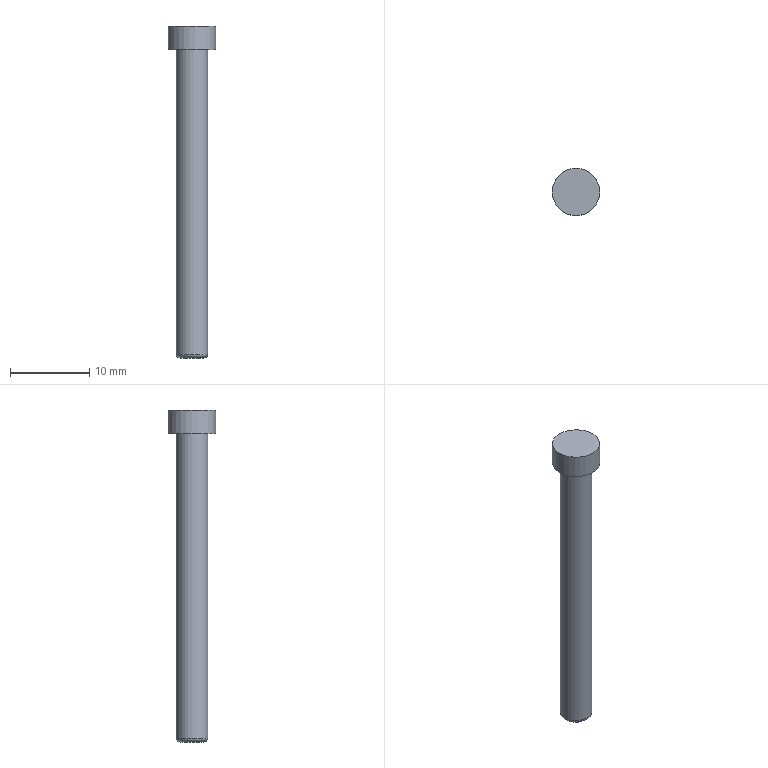Part | STEP file | gslz 2016.10.28-10_id3150_x_t | 1 solid | 6 faces | box 6 x 6 x 42 mm | volume 574.275 mm3 | plane 3 | cylinder 2 | torus 1 | commonest cylinder face diameters 4 x1 6 x1
STEP:
#1=CARTESIAN_POINT('',(0.,0.,0.));
#2=DIRECTION('',(0.,0.,1.));
#3=DIRECTION('',(1.,0.,0.));
#4=AXIS2_PLACEMENT_3D('',#1,#2,#3);
#5=CARTESIAN_POINT('',(-433.068,149.5,-7.5));
#6=VERTEX_POINT('',#5);
#7=CARTESIAN_POINT('',(-435.068,149.5,-7.5));
#8=DIRECTION('',(0.,0.,1.));
#9=DIRECTION('',(1.,0.,0.));
#10=AXIS2_PLACEMENT_3D('',#7,#8,#9);
#11=CIRCLE('',#10,2.);
#12=CARTESIAN_POINT('',(-435.068,149.5,-6.));
#13=DIRECTION('',(0.,0.,1.));
#14=DIRECTION('',(-1.,0.,0.));
#15=AXIS2_PLACEMENT_3D('',#12,#13,#14);
#16=CYLINDRICAL_SURFACE('',#15,2.);
#17=CARTESIAN_POINT('',(3.142,-1.5));
#18=DIRECTION('',(1.,0.));
#19=VECTOR('',#18,1.);
#20=LINE('',#17,#19);
#21=(GEOMETRIC_REPRESENTATION_CONTEXT(2)PARAMETRIC_REPRESENTATION_CONTEXT()REPRESENTATION_CONTEXT('',''));
#22=DEFINITIONAL_REPRESENTATION('',(#20),#21);
#23=PCURVE('',#16,#22);
#24=CARTESIAN_POINT('',(-435.068,149.5,-7.5));
#25=DIRECTION('',(0.,0.,1.));
#26=DIRECTION('',(-1.,0.,0.));
#27=AXIS2_PLACEMENT_3D('',#24,#25,#26);
#28=TOROIDAL_SURFACE('',#27,1.5,0.5);
#29=CARTESIAN_POINT('',(3.142,6.283));
#30=DIRECTION('',(1.,0.));
#31=VECTOR('',#30,1.);
#32=LINE('',#29,#31);
#33=(GEOMETRIC_REPRESENTATION_CONTEXT(2)PARAMETRIC_REPRESENTATION_CONTEXT()REPRESENTATION_CONTEXT('',''));
#34=DEFINITIONAL_REPRESENTATION('',(#32),#33);
#35=PCURVE('',#28,#34);
#36=SURFACE_CURVE('',#11,(#23,#35),.PCURVE_S1.);
#37=EDGE_CURVE('',#6,#6,#36,.T.);
#38=ORIENTED_EDGE('',*,*,#37,.T.);
#39=CARTESIAN_POINT('',(-433.068,149.5,31.));
#40=VERTEX_POINT('',#39);
#41=CARTESIAN_POINT('',(-433.068,149.5,-7.5));
#42=CARTESIAN_POINT('',(-433.068,149.5,31.));
#43=B_SPLINE_CURVE_WITH_KNOTS('',1,(#41,#42),.UNSPECIFIED.,.F.,.F.,(2,2),(-1.5,37.),.PIECEWISE_BEZIER_KNOTS.);
#44=CARTESIAN_POINT('',(9.425,0.));
#45=DIRECTION('',(0.,1.));
#46=VECTOR('',#45,1.);
#47=LINE('',#44,#46);
#48=(GEOMETRIC_REPRESENTATION_CONTEXT(2)PARAMETRIC_REPRESENTATION_CONTEXT()REPRESENTATION_CONTEXT('',''));
#49=DEFINITIONAL_REPRESENTATION('',(#47),#48);
#50=PCURVE('',#16,#49);
#51=CARTESIAN_POINT('',(3.142,0.));
#52=DIRECTION('',(0.,1.));
#53=VECTOR('',#52,1.);
#54=LINE('',#51,#53);
#55=(GEOMETRIC_REPRESENTATION_CONTEXT(2)PARAMETRIC_REPRESENTATION_CONTEXT()REPRESENTATION_CONTEXT('',''));
#56=DEFINITIONAL_REPRESENTATION('',(#54),#55);
#57=PCURVE('',#16,#56);
#58=SEAM_CURVE('',#43,(#50,#57),.PCURVE_S1.);
#59=EDGE_CURVE('',#6,#40,#58,.T.);
#60=ORIENTED_EDGE('',*,*,#59,.T.);
#61=CARTESIAN_POINT('',(-435.068,149.5,31.));
#62=DIRECTION('',(0.,0.,1.));
#63=DIRECTION('',(1.,0.,0.));
#64=AXIS2_PLACEMENT_3D('',#61,#62,#63);
#65=CIRCLE('',#64,2.);
#66=CARTESIAN_POINT('',(3.142,37.));
#67=DIRECTION('',(1.,0.));
#68=VECTOR('',#67,1.);
#69=LINE('',#66,#68);
#70=(GEOMETRIC_REPRESENTATION_CONTEXT(2)PARAMETRIC_REPRESENTATION_CONTEXT()REPRESENTATION_CONTEXT('',''));
#71=DEFINITIONAL_REPRESENTATION('',(#69),#70);
#72=PCURVE('',#16,#71);
#73=CARTESIAN_POINT('',(-435.068,149.5,31.));
#74=DIRECTION('',(0.,0.,1.));
#75=DIRECTION('',(-1.,0.,0.));
#76=AXIS2_PLACEMENT_3D('',#73,#74,#75);
#77=PLANE('',#76);
#78=CARTESIAN_POINT('',(0.,0.));
#79=DIRECTION('',(-1.,0.));
#80=AXIS2_PLACEMENT_2D('',#78,#79);
#81=CIRCLE('',#80,2.);
#82=(GEOMETRIC_REPRESENTATION_CONTEXT(2)PARAMETRIC_REPRESENTATION_CONTEXT()REPRESENTATION_CONTEXT('',''));
#83=DEFINITIONAL_REPRESENTATION('',(#81),#82);
#84=PCURVE('',#77,#83);
#85=SURFACE_CURVE('',#65,(#72,#84),.PCURVE_S1.);
#86=EDGE_CURVE('',#40,#40,#85,.T.);
#87=ORIENTED_EDGE('',*,*,#86,.F.);
#88=ORIENTED_EDGE('',*,*,#59,.F.);
#89=EDGE_LOOP('',(#38,#60,#87,#88));
#90=FACE_BOUND('',#89,.T.);
#91=ADVANCED_FACE('',(#90),#16,.T.);
#92=CARTESIAN_POINT('',(-433.568,149.5,-8.));
#93=VERTEX_POINT('',#92);
#94=CARTESIAN_POINT('',(-435.068,149.5,-8.));
#95=DIRECTION('',(0.,0.,-1.));
#96=DIRECTION('',(1.,0.,0.));
#97=AXIS2_PLACEMENT_3D('',#94,#95,#96);
#98=CIRCLE('',#97,1.5);
#99=CARTESIAN_POINT('',(-435.068,149.5,-8.));
#100=DIRECTION('',(0.,0.,1.));
#101=DIRECTION('',(-1.,0.,0.));
#102=AXIS2_PLACEMENT_3D('',#99,#100,#101);
#103=PLANE('',#102);
#104=CARTESIAN_POINT('',(-1.5,0.));
#105=CARTESIAN_POINT('',(-1.5,2.598));
#106=CARTESIAN_POINT('',(0.75,1.299));
#107=CARTESIAN_POINT('',(3.,0.));
#108=CARTESIAN_POINT('',(0.75,-1.299));
#109=CARTESIAN_POINT('',(-1.5,-2.598));
#110=CARTESIAN_POINT('',(-1.5,0.));
#111=(BOUNDED_CURVE()B_SPLINE_CURVE(2,(#104,#105,#106,#107,#108,#109,#110),.UNSPECIFIED.,.T.,.F.)B_SPLINE_CURVE_WITH_KNOTS((1,2,2,2,2,1),(-2.094,0.,2.094,4.189,6.283,8.378),.UNSPECIFIED.)CURVE()GEOMETRIC_REPRESENTATION_ITEM()RATIONAL_B_SPLINE_CURVE((1.,0.5,1.,0.5,1.,0.5,1.))REPRESENTATION_ITEM(''));
#112=(GEOMETRIC_REPRESENTATION_CONTEXT(2)PARAMETRIC_REPRESENTATION_CONTEXT()REPRESENTATION_CONTEXT('',''));
#113=DEFINITIONAL_REPRESENTATION('',(#111),#112);
#114=PCURVE('',#103,#113);
#115=CARTESIAN_POINT('',(9.425,4.712));
#116=DIRECTION('',(-1.,0.));
#117=VECTOR('',#116,1.);
#118=LINE('',#115,#117);
#119=(GEOMETRIC_REPRESENTATION_CONTEXT(2)PARAMETRIC_REPRESENTATION_CONTEXT()REPRESENTATION_CONTEXT('',''));
#120=DEFINITIONAL_REPRESENTATION('',(#118),#119);
#121=PCURVE('',#28,#120);
#122=SURFACE_CURVE('',#98,(#114,#121),.PCURVE_S1.);
#123=EDGE_CURVE('',#93,#93,#122,.T.);
#124=ORIENTED_EDGE('',*,*,#123,.T.);
#125=EDGE_LOOP('',(#124));
#126=FACE_BOUND('',#125,.T.);
#127=ADVANCED_FACE('',(#126),#103,.F.);
#128=CARTESIAN_POINT('',(-432.068,149.5,31.));
#129=VERTEX_POINT('',#128);
#130=CARTESIAN_POINT('',(-435.068,149.5,31.));
#131=DIRECTION('',(0.,0.,1.));
#132=DIRECTION('',(1.,0.,0.));
#133=AXIS2_PLACEMENT_3D('',#130,#131,#132);
#134=CIRCLE('',#133,3.);
#135=CARTESIAN_POINT('',(0.,0.));
#136=DIRECTION('',(-1.,0.));
#137=AXIS2_PLACEMENT_2D('',#135,#136);
#138=CIRCLE('',#137,3.);
#139=(GEOMETRIC_REPRESENTATION_CONTEXT(2)PARAMETRIC_REPRESENTATION_CONTEXT()REPRESENTATION_CONTEXT('',''));
#140=DEFINITIONAL_REPRESENTATION('',(#138),#139);
#141=PCURVE('',#77,#140);
#142=CARTESIAN_POINT('',(-435.068,149.5,34.));
#143=DIRECTION('',(0.,0.,-1.));
#144=DIRECTION('',(1.,0.,0.));
#145=AXIS2_PLACEMENT_3D('',#142,#143,#144);
#146=CYLINDRICAL_SURFACE('',#145,3.);
#147=CARTESIAN_POINT('',(6.283,3.));
#148=DIRECTION('',(-1.,0.));
#149=VECTOR('',#148,1.);
#150=LINE('',#147,#149);
#151=(GEOMETRIC_REPRESENTATION_CONTEXT(2)PARAMETRIC_REPRESENTATION_CONTEXT()REPRESENTATION_CONTEXT('',''));
#152=DEFINITIONAL_REPRESENTATION('',(#150),#151);
#153=PCURVE('',#146,#152);
#154=SURFACE_CURVE('',#134,(#141,#153),.PCURVE_S1.);
#155=EDGE_CURVE('',#129,#129,#154,.T.);
#156=ORIENTED_EDGE('',*,*,#155,.F.);
#157=EDGE_LOOP('',(#156));
#158=FACE_BOUND('',#157,.T.);
#159=ORIENTED_EDGE('',*,*,#86,.T.);
#160=EDGE_LOOP('',(#159));
#161=FACE_BOUND('',#160,.T.);
#162=ADVANCED_FACE('',(#158,#161),#77,.F.);
#163=CARTESIAN_POINT('',(-432.068,149.5,34.));
#164=VERTEX_POINT('',#163);
#165=CARTESIAN_POINT('',(-435.068,149.5,34.));
#166=DIRECTION('',(0.,0.,1.));
#167=DIRECTION('',(1.,0.,0.));
#168=AXIS2_PLACEMENT_3D('',#165,#166,#167);
#169=CIRCLE('',#168,3.);
#170=CARTESIAN_POINT('',(6.283,0.));
#171=DIRECTION('',(-1.,0.));
#172=VECTOR('',#171,1.);
#173=LINE('',#170,#172);
#174=(GEOMETRIC_REPRESENTATION_CONTEXT(2)PARAMETRIC_REPRESENTATION_CONTEXT()REPRESENTATION_CONTEXT('',''));
#175=DEFINITIONAL_REPRESENTATION('',(#173),#174);
#176=PCURVE('',#146,#175);
#177=CARTESIAN_POINT('',(-435.068,149.5,34.));
#178=DIRECTION('',(0.,0.,1.));
#179=DIRECTION('',(-1.,0.,0.));
#180=AXIS2_PLACEMENT_3D('',#177,#178,#179);
#181=PLANE('',#180);
#182=CARTESIAN_POINT('',(0.,0.));
#183=DIRECTION('',(-1.,0.));
#184=AXIS2_PLACEMENT_2D('',#182,#183);
#185=CIRCLE('',#184,3.);
#186=(GEOMETRIC_REPRESENTATION_CONTEXT(2)PARAMETRIC_REPRESENTATION_CONTEXT()REPRESENTATION_CONTEXT('',''));
#187=DEFINITIONAL_REPRESENTATION('',(#185),#186);
#188=PCURVE('',#181,#187);
#189=SURFACE_CURVE('',#169,(#176,#188),.PCURVE_S1.);
#190=EDGE_CURVE('',#164,#164,#189,.T.);
#191=ORIENTED_EDGE('',*,*,#190,.F.);
#192=CARTESIAN_POINT('',(-432.068,149.5,34.));
#193=CARTESIAN_POINT('',(-432.068,149.5,31.));
#194=B_SPLINE_CURVE_WITH_KNOTS('',1,(#192,#193),.UNSPECIFIED.,.F.,.F.,(2,2),(0.,3.),.PIECEWISE_BEZIER_KNOTS.);
#195=CARTESIAN_POINT('',(6.283,0.));
#196=DIRECTION('',(0.,1.));
#197=VECTOR('',#196,1.);
#198=LINE('',#195,#197);
#199=(GEOMETRIC_REPRESENTATION_CONTEXT(2)PARAMETRIC_REPRESENTATION_CONTEXT()REPRESENTATION_CONTEXT('',''));
#200=DEFINITIONAL_REPRESENTATION('',(#198),#199);
#201=PCURVE('',#146,#200);
#202=CARTESIAN_POINT('',(0.,0.));
#203=DIRECTION('',(0.,1.));
#204=VECTOR('',#203,1.);
#205=LINE('',#202,#204);
#206=(GEOMETRIC_REPRESENTATION_CONTEXT(2)PARAMETRIC_REPRESENTATION_CONTEXT()REPRESENTATION_CONTEXT('',''));
#207=DEFINITIONAL_REPRESENTATION('',(#205),#206);
#208=PCURVE('',#146,#207);
#209=SEAM_CURVE('',#194,(#201,#208),.PCURVE_S1.);
#210=EDGE_CURVE('',#164,#129,#209,.T.);
#211=ORIENTED_EDGE('',*,*,#210,.T.);
#212=ORIENTED_EDGE('',*,*,#155,.T.);
#213=ORIENTED_EDGE('',*,*,#210,.F.);
#214=EDGE_LOOP('',(#191,#211,#212,#213));
#215=FACE_BOUND('',#214,.T.);
#216=ADVANCED_FACE('',(#215),#146,.T.);
#217=ORIENTED_EDGE('',*,*,#190,.T.);
#218=EDGE_LOOP('',(#217));
#219=FACE_BOUND('',#218,.T.);
#220=ADVANCED_FACE('',(#219),#181,.T.);
#221=ORIENTED_EDGE('',*,*,#123,.F.);
#222=CARTESIAN_POINT('',(-433.568,149.5,-8.));
#223=CARTESIAN_POINT('',(-433.434,149.5,-8.));
#224=CARTESIAN_POINT('',(-433.304,149.5,-7.957));
#225=CARTESIAN_POINT('',(-433.192,149.5,-7.876));
#226=CARTESIAN_POINT('',(-433.11,149.5,-7.764));
#227=CARTESIAN_POINT('',(-433.068,149.5,-7.634));
#228=CARTESIAN_POINT('',(-433.068,149.5,-7.5));
#229=(BOUNDED_CURVE()B_SPLINE_CURVE(6,(#222,#223,#224,#225,#226,#227,#228),.UNSPECIFIED.,.F.,.F.)B_SPLINE_CURVE_WITH_KNOTS((7,7),(4.712,6.283),.PIECEWISE_BEZIER_KNOTS.)CURVE()GEOMETRIC_REPRESENTATION_ITEM()RATIONAL_B_SPLINE_CURVE((1.031,1.01,0.9979,0.994,0.9979,1.01,1.031))REPRESENTATION_ITEM(''));
#230=CARTESIAN_POINT('',(9.425,0.));
#231=DIRECTION('',(0.,1.));
#232=VECTOR('',#231,1.);
#233=LINE('',#230,#232);
#234=(GEOMETRIC_REPRESENTATION_CONTEXT(2)PARAMETRIC_REPRESENTATION_CONTEXT()REPRESENTATION_CONTEXT('',''));
#235=DEFINITIONAL_REPRESENTATION('',(#233),#234);
#236=PCURVE('',#28,#235);
#237=CARTESIAN_POINT('',(3.142,0.));
#238=DIRECTION('',(0.,1.));
#239=VECTOR('',#238,1.);
#240=LINE('',#237,#239);
#241=(GEOMETRIC_REPRESENTATION_CONTEXT(2)PARAMETRIC_REPRESENTATION_CONTEXT()REPRESENTATION_CONTEXT('',''));
#242=DEFINITIONAL_REPRESENTATION('',(#240),#241);
#243=PCURVE('',#28,#242);
#244=SEAM_CURVE('',#229,(#236,#243),.PCURVE_S1.);
#245=EDGE_CURVE('',#93,#6,#244,.T.);
#246=ORIENTED_EDGE('',*,*,#245,.T.);
#247=ORIENTED_EDGE('',*,*,#37,.F.);
#248=ORIENTED_EDGE('',*,*,#245,.F.);
#249=EDGE_LOOP('',(#221,#246,#247,#248));
#250=FACE_BOUND('',#249,.T.);
#251=ADVANCED_FACE('',(#250),#28,.T.);
#252=CLOSED_SHELL('',(#91,#127,#162,#216,#220,#251));
#253=MANIFOLD_SOLID_BREP('',#252);
#254=(LENGTH_UNIT()NAMED_UNIT(*)SI_UNIT(.MILLI.,.METRE.));
#255=UNCERTAINTY_MEASURE_WITH_UNIT(LENGTH_MEASURE(0.00001),#254,'','');
#256=(NAMED_UNIT(*)PLANE_ANGLE_UNIT()SI_UNIT($,.RADIAN.));
#257=(NAMED_UNIT(*)SI_UNIT($,.STERADIAN.)SOLID_ANGLE_UNIT());
#258=(GEOMETRIC_REPRESENTATION_CONTEXT(3)GLOBAL_UNCERTAINTY_ASSIGNED_CONTEXT((#255))GLOBAL_UNIT_ASSIGNED_CONTEXT((#254,#256,#257))REPRESENTATION_CONTEXT('',''));
#259=ADVANCED_BREP_SHAPE_REPRESENTATION('',(#4,#253),#258);